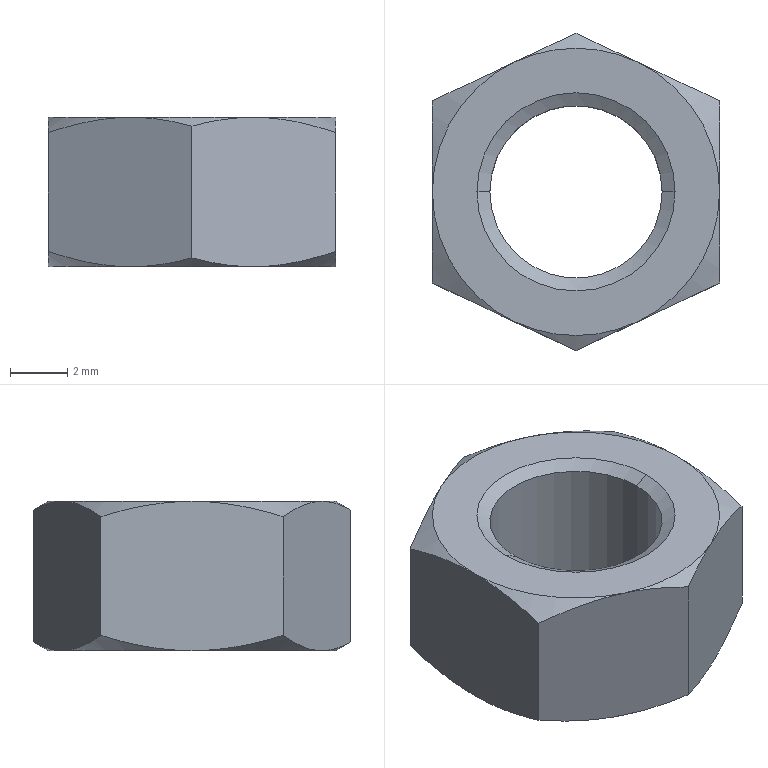Part | SolidWorks | features BaseBody 1 | 1 solid | 26 faces | box 10 x 11.05 x 5.2 mm | volume 300.51 mm3 | cone 16 | plane 8 | cylinder 2 | commonest cylinder face diameters 6 x2
STEP:
#1=CARTESIAN_POINT('',(107.5,-21.,59.86));
#2=VERTEX_POINT('',#1);
#3=CARTESIAN_POINT('',(113.5,-21.,59.86));
#4=VERTEX_POINT('',#3);
#5=CARTESIAN_POINT('',(110.5,-21.,59.86));
#6=DIRECTION('',(0.,0.,1.));
#7=DIRECTION('',(-1.,0.,0.));
#8=AXIS2_PLACEMENT_3D('',#5,#6,#7);
#9=CIRCLE('',#8,3.);
#10=EDGE_CURVE('',#2,#4,#9,.T.);
#11=ORIENTED_EDGE('',*,*,#10,.T.);
#12=CARTESIAN_POINT('',(113.95,-21.,59.6));
#13=VERTEX_POINT('',#12);
#14=CARTESIAN_POINT('',(113.95,-21.,59.6));
#15=DIRECTION('',(0.866,0.,-0.5));
#16=VECTOR('',#15,1000.);
#17=LINE('',#14,#16);
#18=EDGE_CURVE('',#4,#13,#17,.T.);
#19=ORIENTED_EDGE('',*,*,#18,.T.);
#20=CARTESIAN_POINT('',(107.05,-21.,59.6));
#21=VERTEX_POINT('',#20);
#22=CARTESIAN_POINT('',(110.5,-21.,59.6));
#23=DIRECTION('',(0.,0.,-1.));
#24=DIRECTION('',(-1.,0.,0.));
#25=AXIS2_PLACEMENT_3D('',#22,#23,#24);
#26=CIRCLE('',#25,3.45);
#27=EDGE_CURVE('',#13,#21,#26,.T.);
#28=ORIENTED_EDGE('',*,*,#27,.T.);
#29=CARTESIAN_POINT('',(107.05,-21.,59.6));
#30=DIRECTION('',(-0.866,0.,-0.5));
#31=VECTOR('',#30,1000.);
#32=LINE('',#29,#31);
#33=EDGE_CURVE('',#2,#21,#32,.T.);
#34=ORIENTED_EDGE('',*,*,#33,.F.);
#35=EDGE_LOOP('',(#11,#19,#28,#34));
#36=FACE_OUTER_BOUND('',#35,.T.);
#37=CARTESIAN_POINT('',(110.5,-21.,59.6));
#38=DIRECTION('',(0.,0.,-1.));
#39=DIRECTION('',(-1.,0.,0.));
#40=AXIS2_PLACEMENT_3D('',#37,#38,#39);
#41=CONICAL_SURFACE('',#40,3.45,1.047);
#42=ADVANCED_FACE('',(#36),#41,.F.);
#43=CARTESIAN_POINT('',(113.5,-21.,64.54));
#44=VERTEX_POINT('',#43);
#45=CARTESIAN_POINT('',(107.5,-21.,64.54));
#46=VERTEX_POINT('',#45);
#47=CARTESIAN_POINT('',(110.5,-21.,64.54));
#48=DIRECTION('',(0.,0.,-1.));
#49=DIRECTION('',(1.,0.,0.));
#50=AXIS2_PLACEMENT_3D('',#47,#48,#49);
#51=CIRCLE('',#50,3.);
#52=EDGE_CURVE('',#44,#46,#51,.T.);
#53=ORIENTED_EDGE('',*,*,#52,.T.);
#54=CARTESIAN_POINT('',(107.05,-21.,64.8));
#55=VERTEX_POINT('',#54);
#56=CARTESIAN_POINT('',(107.05,-21.,64.8));
#57=DIRECTION('',(-0.866,0.,0.5));
#58=VECTOR('',#57,1000.);
#59=LINE('',#56,#58);
#60=EDGE_CURVE('',#46,#55,#59,.T.);
#61=ORIENTED_EDGE('',*,*,#60,.T.);
#62=CARTESIAN_POINT('',(113.95,-21.,64.8));
#63=VERTEX_POINT('',#62);
#64=CARTESIAN_POINT('',(110.5,-21.,64.8));
#65=DIRECTION('',(0.,0.,1.));
#66=DIRECTION('',(1.,0.,0.));
#67=AXIS2_PLACEMENT_3D('',#64,#65,#66);
#68=CIRCLE('',#67,3.45);
#69=EDGE_CURVE('',#55,#63,#68,.T.);
#70=ORIENTED_EDGE('',*,*,#69,.T.);
#71=CARTESIAN_POINT('',(113.95,-21.,64.8));
#72=DIRECTION('',(0.866,0.,0.5));
#73=VECTOR('',#72,1000.);
#74=LINE('',#71,#73);
#75=EDGE_CURVE('',#44,#63,#74,.T.);
#76=ORIENTED_EDGE('',*,*,#75,.F.);
#77=EDGE_LOOP('',(#53,#61,#70,#76));
#78=FACE_OUTER_BOUND('',#77,.T.);
#79=CARTESIAN_POINT('',(110.5,-21.,64.8));
#80=DIRECTION('',(0.,0.,1.));
#81=DIRECTION('',(1.,0.,0.));
#82=AXIS2_PLACEMENT_3D('',#79,#80,#81);
#83=CONICAL_SURFACE('',#82,3.45,1.047);
#84=ADVANCED_FACE('',(#78),#83,.F.);
#85=ORIENTED_EDGE('',*,*,#52,.F.);
#86=CARTESIAN_POINT('',(113.5,-21.,64.8));
#87=DIRECTION('',(0.,0.,-1.));
#88=VECTOR('',#87,1000.);
#89=LINE('',#86,#88);
#90=EDGE_CURVE('',#44,#4,#89,.T.);
#91=ORIENTED_EDGE('',*,*,#90,.T.);
#92=ORIENTED_EDGE('',*,*,#10,.F.);
#93=CARTESIAN_POINT('',(107.5,-21.,64.8));
#94=DIRECTION('',(0.,0.,-1.));
#95=VECTOR('',#94,1000.);
#96=LINE('',#93,#95);
#97=EDGE_CURVE('',#46,#2,#96,.T.);
#98=ORIENTED_EDGE('',*,*,#97,.F.);
#99=EDGE_LOOP('',(#85,#91,#92,#98));
#100=FACE_OUTER_BOUND('',#99,.T.);
#101=CARTESIAN_POINT('',(110.5,-21.,64.8));
#102=DIRECTION('',(0.,0.,-1.));
#103=DIRECTION('',(-1.,0.,0.));
#104=AXIS2_PLACEMENT_3D('',#101,#102,#103);
#105=CYLINDRICAL_SURFACE('',#104,3.);
#106=ADVANCED_FACE('',(#100),#105,.F.);
#107=CARTESIAN_POINT('',(110.5,-15.475,64.497));
#108=VERTEX_POINT('',#107);
#109=CARTESIAN_POINT('',(108.373,-16.475,64.8));
#110=VERTEX_POINT('',#109);
#111=CARTESIAN_POINT('',(110.5,-15.475,64.497));
#112=CARTESIAN_POINT('',(109.799,-15.805,64.687));
#113=CARTESIAN_POINT('',(109.09,-16.138,64.8));
#114=CARTESIAN_POINT('',(108.373,-16.475,64.8));
#115=B_SPLINE_CURVE_WITH_KNOTS('',3,(#111,#112,#113,#114),.UNSPECIFIED.,.F.,.F.,(4,4),(0.000000225,0.002369),.UNSPECIFIED.);
#116=EDGE_CURVE('',#108,#110,#115,.T.);
#117=ORIENTED_EDGE('',*,*,#116,.F.);
#118=CARTESIAN_POINT('',(110.5,-15.475,59.903));
#119=VERTEX_POINT('',#118);
#120=CARTESIAN_POINT('',(110.5,-15.475,64.8));
#121=DIRECTION('',(0.,0.,-1.));
#122=VECTOR('',#121,1000.);
#123=LINE('',#120,#122);
#124=EDGE_CURVE('',#108,#119,#123,.T.);
#125=ORIENTED_EDGE('',*,*,#124,.T.);
#126=CARTESIAN_POINT('',(108.373,-16.475,59.6));
#127=VERTEX_POINT('',#126);
#128=CARTESIAN_POINT('',(108.373,-16.475,59.6));
#129=CARTESIAN_POINT('',(109.094,-16.136,59.6));
#130=CARTESIAN_POINT('',(109.801,-15.804,59.713));
#131=CARTESIAN_POINT('',(110.5,-15.475,59.903));
#132=B_SPLINE_CURVE_WITH_KNOTS('',3,(#128,#129,#130,#131),.UNSPECIFIED.,.F.,.F.,(4,4),(0.003219,0.005576),.UNSPECIFIED.);
#133=EDGE_CURVE('',#127,#119,#132,.T.);
#134=ORIENTED_EDGE('',*,*,#133,.F.);
#135=CARTESIAN_POINT('',(105.5,-17.826,60.133));
#136=VERTEX_POINT('',#135);
#137=CARTESIAN_POINT('',(105.5,-17.826,60.133));
#138=CARTESIAN_POINT('',(106.436,-17.386,59.813));
#139=CARTESIAN_POINT('',(107.389,-16.938,59.6));
#140=CARTESIAN_POINT('',(108.373,-16.475,59.6));
#141=B_SPLINE_CURVE_WITH_KNOTS('',3,(#137,#138,#139,#140),.UNSPECIFIED.,.F.,.F.,(4,4),(0.000000229,0.003219),.UNSPECIFIED.);
#142=EDGE_CURVE('',#136,#127,#141,.T.);
#143=ORIENTED_EDGE('',*,*,#142,.F.);
#144=CARTESIAN_POINT('',(105.5,-17.826,64.267));
#145=VERTEX_POINT('',#144);
#146=CARTESIAN_POINT('',(105.5,-17.826,64.8));
#147=DIRECTION('',(0.,0.,-1.));
#148=VECTOR('',#147,1000.);
#149=LINE('',#146,#148);
#150=EDGE_CURVE('',#145,#136,#149,.T.);
#151=ORIENTED_EDGE('',*,*,#150,.F.);
#152=CARTESIAN_POINT('',(108.373,-16.475,64.8));
#153=CARTESIAN_POINT('',(108.13,-16.589,64.8));
#154=CARTESIAN_POINT('',(107.885,-16.704,64.787));
#155=CARTESIAN_POINT('',(107.398,-16.933,64.738));
#156=CARTESIAN_POINT('',(107.157,-17.047,64.701));
#157=CARTESIAN_POINT('',(106.439,-17.384,64.561));
#158=CARTESIAN_POINT('',(105.967,-17.606,64.427));
#159=CARTESIAN_POINT('',(105.5,-17.826,64.267));
#160=B_SPLINE_CURVE_WITH_KNOTS('',3,(#152,#153,#154,#155,#156,#157,#158,#159),.UNSPECIFIED.,.F.,.F.,(4,2,2,4),(0.002369,0.00317,0.003971,0.005574),.UNSPECIFIED.);
#161=EDGE_CURVE('',#110,#145,#160,.T.);
#162=ORIENTED_EDGE('',*,*,#161,.F.);
#163=EDGE_LOOP('',(#117,#125,#134,#143,#151,#162));
#164=FACE_OUTER_BOUND('',#163,.T.);
#165=CARTESIAN_POINT('',(105.5,-17.826,64.8));
#166=DIRECTION('',(0.4255,-0.905,0.));
#167=DIRECTION('',(0.905,0.4255,0.));
#168=AXIS2_PLACEMENT_3D('',#165,#166,#167);
#169=PLANE('',#168);
#170=ADVANCED_FACE('',(#164),#169,.F.);
#171=CARTESIAN_POINT('',(105.5,-21.,64.8));
#172=VERTEX_POINT('',#171);
#173=CARTESIAN_POINT('',(105.5,-17.826,64.267));
#174=CARTESIAN_POINT('',(105.5,-18.34,64.427));
#175=CARTESIAN_POINT('',(105.5,-18.861,64.56));
#176=CARTESIAN_POINT('',(105.5,-19.654,64.701));
#177=CARTESIAN_POINT('',(105.5,-19.92,64.737));
#178=CARTESIAN_POINT('',(105.5,-20.458,64.787));
#179=CARTESIAN_POINT('',(105.5,-20.73,64.8));
#180=CARTESIAN_POINT('',(105.5,-21.,64.8));
#181=B_SPLINE_CURVE_WITH_KNOTS('',3,(#173,#174,#175,#176,#177,#178,#179,#180),.UNSPECIFIED.,.F.,.F.,(4,2,2,4),(0.01571,0.01731,0.01812,0.01892),.UNSPECIFIED.);
#182=EDGE_CURVE('',#145,#172,#181,.T.);
#183=ORIENTED_EDGE('',*,*,#182,.F.);
#184=ORIENTED_EDGE('',*,*,#150,.T.);
#185=CARTESIAN_POINT('',(105.5,-21.,59.6));
#186=VERTEX_POINT('',#185);
#187=CARTESIAN_POINT('',(105.5,-21.,59.6));
#188=CARTESIAN_POINT('',(105.5,-20.73,59.6));
#189=CARTESIAN_POINT('',(105.5,-20.458,59.613));
#190=CARTESIAN_POINT('',(105.5,-19.92,59.663));
#191=CARTESIAN_POINT('',(105.5,-19.654,59.699));
#192=CARTESIAN_POINT('',(105.5,-18.861,59.84));
#193=CARTESIAN_POINT('',(105.5,-18.34,59.973));
#194=CARTESIAN_POINT('',(105.5,-17.826,60.133));
#195=B_SPLINE_CURVE_WITH_KNOTS('',3,(#187,#188,#189,#190,#191,#192,#193,#194),.UNSPECIFIED.,.F.,.F.,(4,2,2,4),(0.008694,0.009499,0.0103,0.01192),.UNSPECIFIED.);
#196=EDGE_CURVE('',#186,#136,#195,.T.);
#197=ORIENTED_EDGE('',*,*,#196,.F.);
#198=CARTESIAN_POINT('',(105.5,-24.174,60.133));
#199=VERTEX_POINT('',#198);
#200=CARTESIAN_POINT('',(105.5,-24.174,60.133));
#201=CARTESIAN_POINT('',(105.5,-23.659,59.973));
#202=CARTESIAN_POINT('',(105.5,-23.132,59.838));
#203=CARTESIAN_POINT('',(105.5,-22.074,59.651));
#204=CARTESIAN_POINT('',(105.5,-21.54,59.6));
#205=CARTESIAN_POINT('',(105.5,-21.,59.6));
#206=B_SPLINE_CURVE_WITH_KNOTS('',3,(#200,#201,#202,#203,#204,#205),.UNSPECIFIED.,.F.,.F.,(4,2,4),(0.00547,0.007082,0.008694),.UNSPECIFIED.);
#207=EDGE_CURVE('',#199,#186,#206,.T.);
#208=ORIENTED_EDGE('',*,*,#207,.F.);
#209=CARTESIAN_POINT('',(105.5,-24.174,64.267));
#210=VERTEX_POINT('',#209);
#211=CARTESIAN_POINT('',(105.5,-24.174,64.8));
#212=DIRECTION('',(0.,0.,-1.));
#213=VECTOR('',#212,1000.);
#214=LINE('',#211,#213);
#215=EDGE_CURVE('',#210,#199,#214,.T.);
#216=ORIENTED_EDGE('',*,*,#215,.F.);
#217=CARTESIAN_POINT('',(105.5,-21.,64.8));
#218=CARTESIAN_POINT('',(105.5,-21.54,64.8));
#219=CARTESIAN_POINT('',(105.5,-22.074,64.749));
#220=CARTESIAN_POINT('',(105.5,-23.132,64.562));
#221=CARTESIAN_POINT('',(105.5,-23.659,64.427));
#222=CARTESIAN_POINT('',(105.5,-24.174,64.267));
#223=B_SPLINE_CURVE_WITH_KNOTS('',3,(#217,#218,#219,#220,#221,#222),.UNSPECIFIED.,.F.,.F.,(4,2,4),(0.01892,0.02053,0.02214),.UNSPECIFIED.);
#224=EDGE_CURVE('',#172,#210,#223,.T.);
#225=ORIENTED_EDGE('',*,*,#224,.F.);
#226=EDGE_LOOP('',(#183,#184,#197,#208,#216,#225));
#227=FACE_OUTER_BOUND('',#226,.T.);
#228=CARTESIAN_POINT('',(105.5,-24.174,64.8));
#229=DIRECTION('',(1.,0.,0.));
#230=DIRECTION('',(0.,0.,-1.));
#231=AXIS2_PLACEMENT_3D('',#228,#229,#230);
#232=PLANE('',#231);
#233=ADVANCED_FACE('',(#227),#232,.F.);
#234=CARTESIAN_POINT('',(108.373,-25.525,64.8));
#235=VERTEX_POINT('',#234);
#236=CARTESIAN_POINT('',(105.5,-24.174,64.267));
#237=CARTESIAN_POINT('',(106.436,-24.614,64.587));
#238=CARTESIAN_POINT('',(107.389,-25.062,64.8));
#239=CARTESIAN_POINT('',(108.373,-25.525,64.8));
#240=B_SPLINE_CURVE_WITH_KNOTS('',3,(#236,#237,#238,#239),.UNSPECIFIED.,.F.,.F.,(4,4),(0.000000229,0.003219),.UNSPECIFIED.);
#241=EDGE_CURVE('',#210,#235,#240,.T.);
#242=ORIENTED_EDGE('',*,*,#241,.F.);
#243=ORIENTED_EDGE('',*,*,#215,.T.);
#244=CARTESIAN_POINT('',(108.373,-25.525,59.6));
#245=VERTEX_POINT('',#244);
#246=CARTESIAN_POINT('',(108.373,-25.525,59.6));
#247=CARTESIAN_POINT('',(108.13,-25.411,59.6));
#248=CARTESIAN_POINT('',(107.885,-25.296,59.613));
#249=CARTESIAN_POINT('',(107.398,-25.067,59.662));
#250=CARTESIAN_POINT('',(107.157,-24.953,59.699));
#251=CARTESIAN_POINT('',(106.439,-24.616,59.839));
#252=CARTESIAN_POINT('',(105.967,-24.394,59.973));
#253=CARTESIAN_POINT('',(105.5,-24.174,60.133));
#254=B_SPLINE_CURVE_WITH_KNOTS('',3,(#246,#247,#248,#249,#250,#251,#252,#253),.UNSPECIFIED.,.F.,.F.,(4,2,2,4),(0.002369,0.00317,0.003971,0.005574),.UNSPECIFIED.);
#255=EDGE_CURVE('',#245,#199,#254,.T.);
#256=ORIENTED_EDGE('',*,*,#255,.F.);
#257=CARTESIAN_POINT('',(110.5,-26.525,59.903));
#258=VERTEX_POINT('',#257);
#259=CARTESIAN_POINT('',(110.5,-26.525,59.903));
#260=CARTESIAN_POINT('',(109.799,-26.195,59.713));
#261=CARTESIAN_POINT('',(109.09,-25.862,59.6));
#262=CARTESIAN_POINT('',(108.373,-25.525,59.6));
#263=B_SPLINE_CURVE_WITH_KNOTS('',3,(#259,#260,#261,#262),.UNSPECIFIED.,.F.,.F.,(4,4),(0.000000225,0.002369),.UNSPECIFIED.);
#264=EDGE_CURVE('',#258,#245,#263,.T.);
#265=ORIENTED_EDGE('',*,*,#264,.F.);
#266=CARTESIAN_POINT('',(110.5,-26.525,64.497));
#267=VERTEX_POINT('',#266);
#268=CARTESIAN_POINT('',(110.5,-26.525,64.8));
#269=DIRECTION('',(0.,0.,-1.));
#270=VECTOR('',#269,1000.);
#271=LINE('',#268,#270);
#272=EDGE_CURVE('',#267,#258,#271,.T.);
#273=ORIENTED_EDGE('',*,*,#272,.F.);
#274=CARTESIAN_POINT('',(108.373,-25.525,64.8));
#275=CARTESIAN_POINT('',(109.094,-25.864,64.8));
#276=CARTESIAN_POINT('',(109.801,-26.196,64.687));
#277=CARTESIAN_POINT('',(110.5,-26.525,64.497));
#278=B_SPLINE_CURVE_WITH_KNOTS('',3,(#274,#275,#276,#277),.UNSPECIFIED.,.F.,.F.,(4,4),(0.003219,0.005576),.UNSPECIFIED.);
#279=EDGE_CURVE('',#235,#267,#278,.T.);
#280=ORIENTED_EDGE('',*,*,#279,.F.);
#281=EDGE_LOOP('',(#242,#243,#256,#265,#273,#280));
#282=FACE_OUTER_BOUND('',#281,.T.);
#283=CARTESIAN_POINT('',(105.5,-24.174,64.8));
#284=DIRECTION('',(0.4255,0.905,0.));
#285=DIRECTION('',(-0.905,0.4255,0.));
#286=AXIS2_PLACEMENT_3D('',#283,#284,#285);
#287=PLANE('',#286);
#288=ADVANCED_FACE('',(#282),#287,.F.);
#289=CARTESIAN_POINT('',(112.627,-25.525,64.8));
#290=VERTEX_POINT('',#289);
#291=CARTESIAN_POINT('',(110.5,-26.525,64.497));
#292=CARTESIAN_POINT('',(111.201,-26.195,64.687));
#293=CARTESIAN_POINT('',(111.91,-25.862,64.8));
#294=CARTESIAN_POINT('',(112.627,-25.525,64.8));
#295=B_SPLINE_CURVE_WITH_KNOTS('',3,(#291,#292,#293,#294),.UNSPECIFIED.,.F.,.F.,(4,4),(0.000000225,0.002369),.UNSPECIFIED.);
#296=EDGE_CURVE('',#267,#290,#295,.T.);
#297=ORIENTED_EDGE('',*,*,#296,.F.);
#298=ORIENTED_EDGE('',*,*,#272,.T.);
#299=CARTESIAN_POINT('',(112.627,-25.525,59.6));
#300=VERTEX_POINT('',#299);
#301=CARTESIAN_POINT('',(112.627,-25.525,59.6));
#302=CARTESIAN_POINT('',(111.906,-25.864,59.6));
#303=CARTESIAN_POINT('',(111.199,-26.196,59.713));
#304=CARTESIAN_POINT('',(110.5,-26.525,59.903));
#305=B_SPLINE_CURVE_WITH_KNOTS('',3,(#301,#302,#303,#304),.UNSPECIFIED.,.F.,.F.,(4,4),(0.003219,0.005576),.UNSPECIFIED.);
#306=EDGE_CURVE('',#300,#258,#305,.T.);
#307=ORIENTED_EDGE('',*,*,#306,.F.);
#308=CARTESIAN_POINT('',(115.5,-24.174,60.133));
#309=VERTEX_POINT('',#308);
#310=CARTESIAN_POINT('',(115.5,-24.174,60.133));
#311=CARTESIAN_POINT('',(114.564,-24.614,59.813));
#312=CARTESIAN_POINT('',(113.611,-25.062,59.6));
#313=CARTESIAN_POINT('',(112.627,-25.525,59.6));
#314=B_SPLINE_CURVE_WITH_KNOTS('',3,(#310,#311,#312,#313),.UNSPECIFIED.,.F.,.F.,(4,4),(0.000000229,0.003219),.UNSPECIFIED.);
#315=EDGE_CURVE('',#309,#300,#314,.T.);
#316=ORIENTED_EDGE('',*,*,#315,.F.);
#317=CARTESIAN_POINT('',(115.5,-24.174,64.267));
#318=VERTEX_POINT('',#317);
#319=CARTESIAN_POINT('',(115.5,-24.174,64.8));
#320=DIRECTION('',(0.,0.,-1.));
#321=VECTOR('',#320,1000.);
#322=LINE('',#319,#321);
#323=EDGE_CURVE('',#318,#309,#322,.T.);
#324=ORIENTED_EDGE('',*,*,#323,.F.);
#325=CARTESIAN_POINT('',(112.627,-25.525,64.8));
#326=CARTESIAN_POINT('',(112.87,-25.411,64.8));
#327=CARTESIAN_POINT('',(113.115,-25.296,64.787));
#328=CARTESIAN_POINT('',(113.602,-25.067,64.738));
#329=CARTESIAN_POINT('',(113.843,-24.953,64.701));
#330=CARTESIAN_POINT('',(114.561,-24.616,64.561));
#331=CARTESIAN_POINT('',(115.033,-24.394,64.427));
#332=CARTESIAN_POINT('',(115.5,-24.174,64.267));
#333=B_SPLINE_CURVE_WITH_KNOTS('',3,(#325,#326,#327,#328,#329,#330,#331,#332),.UNSPECIFIED.,.F.,.F.,(4,2,2,4),(0.002369,0.00317,0.003971,0.005574),.UNSPECIFIED.);
#334=EDGE_CURVE('',#290,#318,#333,.T.);
#335=ORIENTED_EDGE('',*,*,#334,.F.);
#336=EDGE_LOOP('',(#297,#298,#307,#316,#324,#335));
#337=FACE_OUTER_BOUND('',#336,.T.);
#338=CARTESIAN_POINT('',(115.5,-24.174,64.8));
#339=DIRECTION('',(-0.4255,0.905,0.));
#340=DIRECTION('',(-0.905,-0.4255,0.));
#341=AXIS2_PLACEMENT_3D('',#338,#339,#340);
#342=PLANE('',#341);
#343=ADVANCED_FACE('',(#337),#342,.F.);
#344=CARTESIAN_POINT('',(115.5,-21.,64.8));
#345=VERTEX_POINT('',#344);
#346=CARTESIAN_POINT('',(115.5,-24.174,64.267));
#347=CARTESIAN_POINT('',(115.5,-23.659,64.427));
#348=CARTESIAN_POINT('',(115.5,-23.132,64.562));
#349=CARTESIAN_POINT('',(115.5,-22.074,64.749));
#350=CARTESIAN_POINT('',(115.5,-21.54,64.8));
#351=CARTESIAN_POINT('',(115.5,-21.,64.8));
#352=B_SPLINE_CURVE_WITH_KNOTS('',3,(#346,#347,#348,#349,#350,#351),.UNSPECIFIED.,.F.,.F.,(4,2,4),(0.00547,0.007082,0.008694),.UNSPECIFIED.);
#353=EDGE_CURVE('',#318,#345,#352,.T.);
#354=ORIENTED_EDGE('',*,*,#353,.F.);
#355=ORIENTED_EDGE('',*,*,#323,.T.);
#356=CARTESIAN_POINT('',(115.5,-21.,59.6));
#357=VERTEX_POINT('',#356);
#358=CARTESIAN_POINT('',(115.5,-21.,59.6));
#359=CARTESIAN_POINT('',(115.5,-21.54,59.6));
#360=CARTESIAN_POINT('',(115.5,-22.074,59.651));
#361=CARTESIAN_POINT('',(115.5,-23.132,59.838));
#362=CARTESIAN_POINT('',(115.5,-23.659,59.973));
#363=CARTESIAN_POINT('',(115.5,-24.174,60.133));
#364=B_SPLINE_CURVE_WITH_KNOTS('',3,(#358,#359,#360,#361,#362,#363),.UNSPECIFIED.,.F.,.F.,(4,2,4),(0.01892,0.02053,0.02214),.UNSPECIFIED.);
#365=EDGE_CURVE('',#357,#309,#364,.T.);
#366=ORIENTED_EDGE('',*,*,#365,.F.);
#367=CARTESIAN_POINT('',(115.5,-17.826,60.133));
#368=VERTEX_POINT('',#367);
#369=CARTESIAN_POINT('',(115.5,-17.826,60.133));
#370=CARTESIAN_POINT('',(115.5,-18.34,59.973));
#371=CARTESIAN_POINT('',(115.5,-18.861,59.84));
#372=CARTESIAN_POINT('',(115.5,-19.654,59.699));
#373=CARTESIAN_POINT('',(115.5,-19.92,59.663));
#374=CARTESIAN_POINT('',(115.5,-20.458,59.613));
#375=CARTESIAN_POINT('',(115.5,-20.73,59.6));
#376=CARTESIAN_POINT('',(115.5,-21.,59.6));
#377=B_SPLINE_CURVE_WITH_KNOTS('',3,(#369,#370,#371,#372,#373,#374,#375,#376),.UNSPECIFIED.,.F.,.F.,(4,2,2,4),(0.01571,0.01731,0.01812,0.01892),.UNSPECIFIED.);
#378=EDGE_CURVE('',#368,#357,#377,.T.);
#379=ORIENTED_EDGE('',*,*,#378,.F.);
#380=CARTESIAN_POINT('',(115.5,-17.826,64.267));
#381=VERTEX_POINT('',#380);
#382=CARTESIAN_POINT('',(115.5,-17.826,64.8));
#383=DIRECTION('',(0.,0.,-1.));
#384=VECTOR('',#383,1000.);
#385=LINE('',#382,#384);
#386=EDGE_CURVE('',#381,#368,#385,.T.);
#387=ORIENTED_EDGE('',*,*,#386,.F.);
#388=CARTESIAN_POINT('',(115.5,-21.,64.8));
#389=CARTESIAN_POINT('',(115.5,-20.73,64.8));
#390=CARTESIAN_POINT('',(115.5,-20.458,64.787));
#391=CARTESIAN_POINT('',(115.5,-19.92,64.737));
#392=CARTESIAN_POINT('',(115.5,-19.654,64.701));
#393=CARTESIAN_POINT('',(115.5,-18.861,64.56));
#394=CARTESIAN_POINT('',(115.5,-18.34,64.427));
#395=CARTESIAN_POINT('',(115.5,-17.826,64.267));
#396=B_SPLINE_CURVE_WITH_KNOTS('',3,(#388,#389,#390,#391,#392,#393,#394,#395),.UNSPECIFIED.,.F.,.F.,(4,2,2,4),(0.008694,0.009499,0.0103,0.01192),.UNSPECIFIED.);
#397=EDGE_CURVE('',#345,#381,#396,.T.);
#398=ORIENTED_EDGE('',*,*,#397,.F.);
#399=EDGE_LOOP('',(#354,#355,#366,#379,#387,#398));
#400=FACE_OUTER_BOUND('',#399,.T.);
#401=CARTESIAN_POINT('',(115.5,-24.174,64.8));
#402=DIRECTION('',(-1.,0.,0.));
#403=DIRECTION('',(0.,0.,1.));
#404=AXIS2_PLACEMENT_3D('',#401,#402,#403);
#405=PLANE('',#404);
#406=ADVANCED_FACE('',(#400),#405,.F.);
#407=CARTESIAN_POINT('',(112.627,-16.475,64.8));
#408=VERTEX_POINT('',#407);
#409=CARTESIAN_POINT('',(115.5,-17.826,64.267));
#410=CARTESIAN_POINT('',(114.564,-17.386,64.587));
#411=CARTESIAN_POINT('',(113.611,-16.938,64.8));
#412=CARTESIAN_POINT('',(112.627,-16.475,64.8));
#413=B_SPLINE_CURVE_WITH_KNOTS('',3,(#409,#410,#411,#412),.UNSPECIFIED.,.F.,.F.,(4,4),(0.000000229,0.003219),.UNSPECIFIED.);
#414=EDGE_CURVE('',#381,#408,#413,.T.);
#415=ORIENTED_EDGE('',*,*,#414,.F.);
#416=ORIENTED_EDGE('',*,*,#386,.T.);
#417=CARTESIAN_POINT('',(112.627,-16.475,59.6));
#418=VERTEX_POINT('',#417);
#419=CARTESIAN_POINT('',(112.627,-16.475,59.6));
#420=CARTESIAN_POINT('',(112.87,-16.589,59.6));
#421=CARTESIAN_POINT('',(113.115,-16.704,59.613));
#422=CARTESIAN_POINT('',(113.602,-16.933,59.662));
#423=CARTESIAN_POINT('',(113.843,-17.047,59.699));
#424=CARTESIAN_POINT('',(114.561,-17.384,59.839));
#425=CARTESIAN_POINT('',(115.033,-17.606,59.973));
#426=CARTESIAN_POINT('',(115.5,-17.826,60.133));
#427=B_SPLINE_CURVE_WITH_KNOTS('',3,(#419,#420,#421,#422,#423,#424,#425,#426),.UNSPECIFIED.,.F.,.F.,(4,2,2,4),(0.002369,0.00317,0.003971,0.005574),.UNSPECIFIED.);
#428=EDGE_CURVE('',#418,#368,#427,.T.);
#429=ORIENTED_EDGE('',*,*,#428,.F.);
#430=CARTESIAN_POINT('',(110.5,-15.475,59.903));
#431=CARTESIAN_POINT('',(111.201,-15.805,59.713));
#432=CARTESIAN_POINT('',(111.91,-16.138,59.6));
#433=CARTESIAN_POINT('',(112.627,-16.475,59.6));
#434=B_SPLINE_CURVE_WITH_KNOTS('',3,(#430,#431,#432,#433),.UNSPECIFIED.,.F.,.F.,(4,4),(0.000000225,0.002369),.UNSPECIFIED.);
#435=EDGE_CURVE('',#119,#418,#434,.T.);
#436=ORIENTED_EDGE('',*,*,#435,.F.);
#437=ORIENTED_EDGE('',*,*,#124,.F.);
#438=CARTESIAN_POINT('',(112.627,-16.475,64.8));
#439=CARTESIAN_POINT('',(111.906,-16.136,64.8));
#440=CARTESIAN_POINT('',(111.199,-15.804,64.687));
#441=CARTESIAN_POINT('',(110.5,-15.475,64.497));
#442=B_SPLINE_CURVE_WITH_KNOTS('',3,(#438,#439,#440,#441),.UNSPECIFIED.,.F.,.F.,(4,4),(0.003219,0.005576),.UNSPECIFIED.);
#443=EDGE_CURVE('',#408,#108,#442,.T.);
#444=ORIENTED_EDGE('',*,*,#443,.F.);
#445=EDGE_LOOP('',(#415,#416,#429,#436,#437,#444));
#446=FACE_OUTER_BOUND('',#445,.T.);
#447=CARTESIAN_POINT('',(115.5,-17.826,64.8));
#448=DIRECTION('',(-0.4255,-0.905,0.));
#449=DIRECTION('',(0.905,-0.4255,0.));
#450=AXIS2_PLACEMENT_3D('',#447,#448,#449);
#451=PLANE('',#450);
#452=ADVANCED_FACE('',(#446),#451,.F.);
#453=CARTESIAN_POINT('',(110.5,-21.,64.8));
#454=DIRECTION('',(0.,0.,1.));
#455=DIRECTION('',(1.,0.,0.));
#456=AXIS2_PLACEMENT_3D('',#453,#454,#455);
#457=CIRCLE('',#456,3.45);
#458=EDGE_CURVE('',#63,#55,#457,.T.);
#459=ORIENTED_EDGE('',*,*,#458,.F.);
#460=ORIENTED_EDGE('',*,*,#69,.F.);
#461=EDGE_LOOP('',(#459,#460));
#462=FACE_BOUND('',#461,.T.);
#463=CARTESIAN_POINT('',(110.5,-21.,64.8));
#464=DIRECTION('',(0.,0.,1.));
#465=DIRECTION('',(1.,0.,0.));
#466=AXIS2_PLACEMENT_3D('',#463,#464,#465);
#467=CIRCLE('',#466,5.);
#468=EDGE_CURVE('',#290,#345,#467,.T.);
#469=ORIENTED_EDGE('',*,*,#468,.T.);
#470=CARTESIAN_POINT('',(110.5,-21.,64.8));
#471=DIRECTION('',(0.,0.,1.));
#472=DIRECTION('',(1.,0.,0.));
#473=AXIS2_PLACEMENT_3D('',#470,#471,#472);
#474=CIRCLE('',#473,5.);
#475=EDGE_CURVE('',#345,#408,#474,.T.);
#476=ORIENTED_EDGE('',*,*,#475,.T.);
#477=CARTESIAN_POINT('',(110.5,-21.,64.8));
#478=DIRECTION('',(0.,0.,1.));
#479=DIRECTION('',(1.,0.,0.));
#480=AXIS2_PLACEMENT_3D('',#477,#478,#479);
#481=CIRCLE('',#480,5.);
#482=EDGE_CURVE('',#408,#110,#481,.T.);
#483=ORIENTED_EDGE('',*,*,#482,.T.);
#484=CARTESIAN_POINT('',(110.5,-21.,64.8));
#485=DIRECTION('',(0.,0.,1.));
#486=DIRECTION('',(1.,0.,0.));
#487=AXIS2_PLACEMENT_3D('',#484,#485,#486);
#488=CIRCLE('',#487,5.);
#489=EDGE_CURVE('',#110,#172,#488,.T.);
#490=ORIENTED_EDGE('',*,*,#489,.T.);
#491=CARTESIAN_POINT('',(110.5,-21.,64.8));
#492=DIRECTION('',(0.,0.,1.));
#493=DIRECTION('',(1.,0.,0.));
#494=AXIS2_PLACEMENT_3D('',#491,#492,#493);
#495=CIRCLE('',#494,5.);
#496=EDGE_CURVE('',#172,#235,#495,.T.);
#497=ORIENTED_EDGE('',*,*,#496,.T.);
#498=CARTESIAN_POINT('',(110.5,-21.,64.8));
#499=DIRECTION('',(0.,0.,1.));
#500=DIRECTION('',(1.,0.,0.));
#501=AXIS2_PLACEMENT_3D('',#498,#499,#500);
#502=CIRCLE('',#501,5.);
#503=EDGE_CURVE('',#235,#290,#502,.T.);
#504=ORIENTED_EDGE('',*,*,#503,.T.);
#505=EDGE_LOOP('',(#469,#476,#483,#490,#497,#504));
#506=FACE_OUTER_BOUND('',#505,.T.);
#507=CARTESIAN_POINT('',(115.5,-13.124,64.8));
#508=DIRECTION('',(0.,0.,1.));
#509=DIRECTION('',(1.,0.,0.));
#510=AXIS2_PLACEMENT_3D('',#507,#508,#509);
#511=PLANE('',#510);
#512=ADVANCED_FACE('',(#462,#506),#511,.T.);
#513=CARTESIAN_POINT('',(110.5,-21.,59.6));
#514=DIRECTION('',(0.,0.,-1.));
#515=DIRECTION('',(-1.,0.,0.));
#516=AXIS2_PLACEMENT_3D('',#513,#514,#515);
#517=CIRCLE('',#516,3.45);
#518=EDGE_CURVE('',#21,#13,#517,.T.);
#519=ORIENTED_EDGE('',*,*,#518,.F.);
#520=ORIENTED_EDGE('',*,*,#27,.F.);
#521=EDGE_LOOP('',(#519,#520));
#522=FACE_BOUND('',#521,.T.);
#523=CARTESIAN_POINT('',(110.5,-21.,59.6));
#524=DIRECTION('',(0.,0.,-1.));
#525=DIRECTION('',(-1.,0.,0.));
#526=AXIS2_PLACEMENT_3D('',#523,#524,#525);
#527=CIRCLE('',#526,5.);
#528=EDGE_CURVE('',#418,#357,#527,.T.);
#529=ORIENTED_EDGE('',*,*,#528,.T.);
#530=CARTESIAN_POINT('',(110.5,-21.,59.6));
#531=DIRECTION('',(0.,0.,-1.));
#532=DIRECTION('',(-1.,0.,0.));
#533=AXIS2_PLACEMENT_3D('',#530,#531,#532);
#534=CIRCLE('',#533,5.);
#535=EDGE_CURVE('',#357,#300,#534,.T.);
#536=ORIENTED_EDGE('',*,*,#535,.T.);
#537=CARTESIAN_POINT('',(110.5,-21.,59.6));
#538=DIRECTION('',(0.,0.,-1.));
#539=DIRECTION('',(-1.,0.,0.));
#540=AXIS2_PLACEMENT_3D('',#537,#538,#539);
#541=CIRCLE('',#540,5.);
#542=EDGE_CURVE('',#300,#245,#541,.T.);
#543=ORIENTED_EDGE('',*,*,#542,.T.);
#544=CARTESIAN_POINT('',(110.5,-21.,59.6));
#545=DIRECTION('',(0.,0.,-1.));
#546=DIRECTION('',(-1.,0.,0.));
#547=AXIS2_PLACEMENT_3D('',#544,#545,#546);
#548=CIRCLE('',#547,5.);
#549=EDGE_CURVE('',#245,#186,#548,.T.);
#550=ORIENTED_EDGE('',*,*,#549,.T.);
#551=CARTESIAN_POINT('',(110.5,-21.,59.6));
#552=DIRECTION('',(0.,0.,-1.));
#553=DIRECTION('',(-1.,0.,0.));
#554=AXIS2_PLACEMENT_3D('',#551,#552,#553);
#555=CIRCLE('',#554,5.);
#556=EDGE_CURVE('',#186,#127,#555,.T.);
#557=ORIENTED_EDGE('',*,*,#556,.T.);
#558=CARTESIAN_POINT('',(110.5,-21.,59.6));
#559=DIRECTION('',(0.,0.,-1.));
#560=DIRECTION('',(-1.,0.,0.));
#561=AXIS2_PLACEMENT_3D('',#558,#559,#560);
#562=CIRCLE('',#561,5.);
#563=EDGE_CURVE('',#127,#418,#562,.T.);
#564=ORIENTED_EDGE('',*,*,#563,.T.);
#565=EDGE_LOOP('',(#529,#536,#543,#550,#557,#564));
#566=FACE_OUTER_BOUND('',#565,.T.);
#567=CARTESIAN_POINT('',(115.5,-13.124,59.6));
#568=DIRECTION('',(0.,0.,1.));
#569=DIRECTION('',(1.,0.,0.));
#570=AXIS2_PLACEMENT_3D('',#567,#568,#569);
#571=PLANE('',#570);
#572=ADVANCED_FACE('',(#522,#566),#571,.F.);
#573=ORIENTED_EDGE('',*,*,#90,.F.);
#574=CARTESIAN_POINT('',(110.5,-21.,64.54));
#575=DIRECTION('',(0.,0.,-1.));
#576=DIRECTION('',(1.,0.,0.));
#577=AXIS2_PLACEMENT_3D('',#574,#575,#576);
#578=CIRCLE('',#577,3.);
#579=EDGE_CURVE('',#46,#44,#578,.T.);
#580=ORIENTED_EDGE('',*,*,#579,.F.);
#581=ORIENTED_EDGE('',*,*,#97,.T.);
#582=CARTESIAN_POINT('',(110.5,-21.,59.86));
#583=DIRECTION('',(0.,0.,1.));
#584=DIRECTION('',(-1.,0.,0.));
#585=AXIS2_PLACEMENT_3D('',#582,#583,#584);
#586=CIRCLE('',#585,3.);
#587=EDGE_CURVE('',#4,#2,#586,.T.);
#588=ORIENTED_EDGE('',*,*,#587,.F.);
#589=EDGE_LOOP('',(#573,#580,#581,#588));
#590=FACE_OUTER_BOUND('',#589,.T.);
#591=CARTESIAN_POINT('',(110.5,-21.,64.8));
#592=DIRECTION('',(0.,0.,-1.));
#593=DIRECTION('',(-1.,0.,0.));
#594=AXIS2_PLACEMENT_3D('',#591,#592,#593);
#595=CYLINDRICAL_SURFACE('',#594,3.);
#596=ADVANCED_FACE('',(#590),#595,.F.);
#597=ORIENTED_EDGE('',*,*,#378,.T.);
#598=ORIENTED_EDGE('',*,*,#528,.F.);
#599=ORIENTED_EDGE('',*,*,#428,.T.);
#600=EDGE_LOOP('',(#597,#598,#599));
#601=FACE_OUTER_BOUND('',#600,.T.);
#602=CARTESIAN_POINT('',(110.5,-21.,59.6));
#603=DIRECTION('',(0.,0.,1.));
#604=DIRECTION('',(-1.,0.,0.));
#605=AXIS2_PLACEMENT_3D('',#602,#603,#604);
#606=CONICAL_SURFACE('',#605,5.,1.047);
#607=ADVANCED_FACE('',(#601),#606,.T.);
#608=ORIENTED_EDGE('',*,*,#133,.T.);
#609=ORIENTED_EDGE('',*,*,#435,.T.);
#610=ORIENTED_EDGE('',*,*,#563,.F.);
#611=EDGE_LOOP('',(#608,#609,#610));
#612=FACE_OUTER_BOUND('',#611,.T.);
#613=CARTESIAN_POINT('',(110.5,-21.,59.6));
#614=DIRECTION('',(0.,0.,1.));
#615=DIRECTION('',(-1.,0.,0.));
#616=AXIS2_PLACEMENT_3D('',#613,#614,#615);
#617=CONICAL_SURFACE('',#616,5.,1.047);
#618=ADVANCED_FACE('',(#612),#617,.T.);
#619=ORIENTED_EDGE('',*,*,#315,.T.);
#620=ORIENTED_EDGE('',*,*,#535,.F.);
#621=ORIENTED_EDGE('',*,*,#365,.T.);
#622=EDGE_LOOP('',(#619,#620,#621));
#623=FACE_OUTER_BOUND('',#622,.T.);
#624=CARTESIAN_POINT('',(110.5,-21.,59.6));
#625=DIRECTION('',(0.,0.,1.));
#626=DIRECTION('',(-1.,0.,0.));
#627=AXIS2_PLACEMENT_3D('',#624,#625,#626);
#628=CONICAL_SURFACE('',#627,5.,1.047);
#629=ADVANCED_FACE('',(#623),#628,.T.);
#630=ORIENTED_EDGE('',*,*,#264,.T.);
#631=ORIENTED_EDGE('',*,*,#542,.F.);
#632=ORIENTED_EDGE('',*,*,#306,.T.);
#633=EDGE_LOOP('',(#630,#631,#632));
#634=FACE_OUTER_BOUND('',#633,.T.);
#635=CARTESIAN_POINT('',(110.5,-21.,59.6));
#636=DIRECTION('',(0.,0.,1.));
#637=DIRECTION('',(-1.,0.,0.));
#638=AXIS2_PLACEMENT_3D('',#635,#636,#637);
#639=CONICAL_SURFACE('',#638,5.,1.047);
#640=ADVANCED_FACE('',(#634),#639,.T.);
#641=ORIENTED_EDGE('',*,*,#255,.T.);
#642=ORIENTED_EDGE('',*,*,#207,.T.);
#643=ORIENTED_EDGE('',*,*,#549,.F.);
#644=EDGE_LOOP('',(#641,#642,#643));
#645=FACE_OUTER_BOUND('',#644,.T.);
#646=CARTESIAN_POINT('',(110.5,-21.,59.6));
#647=DIRECTION('',(0.,0.,1.));
#648=DIRECTION('',(-1.,0.,0.));
#649=AXIS2_PLACEMENT_3D('',#646,#647,#648);
#650=CONICAL_SURFACE('',#649,5.,1.047);
#651=ADVANCED_FACE('',(#645),#650,.T.);
#652=ORIENTED_EDGE('',*,*,#196,.T.);
#653=ORIENTED_EDGE('',*,*,#142,.T.);
#654=ORIENTED_EDGE('',*,*,#556,.F.);
#655=EDGE_LOOP('',(#652,#653,#654));
#656=FACE_OUTER_BOUND('',#655,.T.);
#657=CARTESIAN_POINT('',(110.5,-21.,59.6));
#658=DIRECTION('',(0.,0.,1.));
#659=DIRECTION('',(-1.,0.,0.));
#660=AXIS2_PLACEMENT_3D('',#657,#658,#659);
#661=CONICAL_SURFACE('',#660,5.,1.047);
#662=ADVANCED_FACE('',(#656),#661,.T.);
#663=ORIENTED_EDGE('',*,*,#334,.T.);
#664=ORIENTED_EDGE('',*,*,#353,.T.);
#665=ORIENTED_EDGE('',*,*,#468,.F.);
#666=EDGE_LOOP('',(#663,#664,#665));
#667=FACE_OUTER_BOUND('',#666,.T.);
#668=CARTESIAN_POINT('',(110.5,-21.,64.8));
#669=DIRECTION('',(0.,0.,-1.));
#670=DIRECTION('',(1.,0.,0.));
#671=AXIS2_PLACEMENT_3D('',#668,#669,#670);
#672=CONICAL_SURFACE('',#671,5.,1.047);
#673=ADVANCED_FACE('',(#667),#672,.T.);
#674=ORIENTED_EDGE('',*,*,#279,.T.);
#675=ORIENTED_EDGE('',*,*,#296,.T.);
#676=ORIENTED_EDGE('',*,*,#503,.F.);
#677=EDGE_LOOP('',(#674,#675,#676));
#678=FACE_OUTER_BOUND('',#677,.T.);
#679=CARTESIAN_POINT('',(110.5,-21.,64.8));
#680=DIRECTION('',(0.,0.,-1.));
#681=DIRECTION('',(1.,0.,0.));
#682=AXIS2_PLACEMENT_3D('',#679,#680,#681);
#683=CONICAL_SURFACE('',#682,5.,1.047);
#684=ADVANCED_FACE('',(#678),#683,.T.);
#685=ORIENTED_EDGE('',*,*,#224,.T.);
#686=ORIENTED_EDGE('',*,*,#241,.T.);
#687=ORIENTED_EDGE('',*,*,#496,.F.);
#688=EDGE_LOOP('',(#685,#686,#687));
#689=FACE_OUTER_BOUND('',#688,.T.);
#690=CARTESIAN_POINT('',(110.5,-21.,64.8));
#691=DIRECTION('',(0.,0.,-1.));
#692=DIRECTION('',(1.,0.,0.));
#693=AXIS2_PLACEMENT_3D('',#690,#691,#692);
#694=CONICAL_SURFACE('',#693,5.,1.047);
#695=ADVANCED_FACE('',(#689),#694,.T.);
#696=ORIENTED_EDGE('',*,*,#161,.T.);
#697=ORIENTED_EDGE('',*,*,#182,.T.);
#698=ORIENTED_EDGE('',*,*,#489,.F.);
#699=EDGE_LOOP('',(#696,#697,#698));
#700=FACE_OUTER_BOUND('',#699,.T.);
#701=CARTESIAN_POINT('',(110.5,-21.,64.8));
#702=DIRECTION('',(0.,0.,-1.));
#703=DIRECTION('',(1.,0.,0.));
#704=AXIS2_PLACEMENT_3D('',#701,#702,#703);
#705=CONICAL_SURFACE('',#704,5.,1.047);
#706=ADVANCED_FACE('',(#700),#705,.T.);
#707=ORIENTED_EDGE('',*,*,#116,.T.);
#708=ORIENTED_EDGE('',*,*,#482,.F.);
#709=ORIENTED_EDGE('',*,*,#443,.T.);
#710=EDGE_LOOP('',(#707,#708,#709));
#711=FACE_OUTER_BOUND('',#710,.T.);
#712=CARTESIAN_POINT('',(110.5,-21.,64.8));
#713=DIRECTION('',(0.,0.,-1.));
#714=DIRECTION('',(1.,0.,0.));
#715=AXIS2_PLACEMENT_3D('',#712,#713,#714);
#716=CONICAL_SURFACE('',#715,5.,1.047);
#717=ADVANCED_FACE('',(#711),#716,.T.);
#718=ORIENTED_EDGE('',*,*,#397,.T.);
#719=ORIENTED_EDGE('',*,*,#414,.T.);
#720=ORIENTED_EDGE('',*,*,#475,.F.);
#721=EDGE_LOOP('',(#718,#719,#720));
#722=FACE_OUTER_BOUND('',#721,.T.);
#723=CARTESIAN_POINT('',(110.5,-21.,64.8));
#724=DIRECTION('',(0.,0.,-1.));
#725=DIRECTION('',(1.,0.,0.));
#726=AXIS2_PLACEMENT_3D('',#723,#724,#725);
#727=CONICAL_SURFACE('',#726,5.,1.047);
#728=ADVANCED_FACE('',(#722),#727,.T.);
#729=ORIENTED_EDGE('',*,*,#60,.F.);
#730=ORIENTED_EDGE('',*,*,#579,.T.);
#731=ORIENTED_EDGE('',*,*,#75,.T.);
#732=ORIENTED_EDGE('',*,*,#458,.T.);
#733=EDGE_LOOP('',(#729,#730,#731,#732));
#734=FACE_OUTER_BOUND('',#733,.T.);
#735=CARTESIAN_POINT('',(110.5,-21.,64.8));
#736=DIRECTION('',(0.,0.,1.));
#737=DIRECTION('',(1.,0.,0.));
#738=AXIS2_PLACEMENT_3D('',#735,#736,#737);
#739=CONICAL_SURFACE('',#738,3.45,1.047);
#740=ADVANCED_FACE('',(#734),#739,.F.);
#741=ORIENTED_EDGE('',*,*,#18,.F.);
#742=ORIENTED_EDGE('',*,*,#587,.T.);
#743=ORIENTED_EDGE('',*,*,#33,.T.);
#744=ORIENTED_EDGE('',*,*,#518,.T.);
#745=EDGE_LOOP('',(#741,#742,#743,#744));
#746=FACE_OUTER_BOUND('',#745,.T.);
#747=CARTESIAN_POINT('',(110.5,-21.,59.6));
#748=DIRECTION('',(0.,0.,-1.));
#749=DIRECTION('',(-1.,0.,0.));
#750=AXIS2_PLACEMENT_3D('',#747,#748,#749);
#751=CONICAL_SURFACE('',#750,3.45,1.047);
#752=ADVANCED_FACE('',(#746),#751,.F.);
#753=CLOSED_SHELL('',(#42,#84,#106,#170,#233,#288,#343,#406,#452,#512,#572,#596,#607,#618,#629,#640,#651,#662,#673,#684,#695,#706,#717,#728,#740,#752));
#754=MANIFOLD_SOLID_BREP('',#753);
#755=CARTESIAN_POINT('',(0.,0.,0.));
#756=DIRECTION('',(0.,0.,1.));
#757=DIRECTION('',(1.,0.,0.));
#758=AXIS2_PLACEMENT_3D('',#755,#756,#757);
#759=(LENGTH_UNIT()NAMED_UNIT(*)SI_UNIT(.MILLI.,.METRE.));
#760=UNCERTAINTY_MEASURE_WITH_UNIT(LENGTH_MEASURE(0.00001),#759,'','');
#761=(NAMED_UNIT(*)PLANE_ANGLE_UNIT()SI_UNIT($,.RADIAN.));
#762=(NAMED_UNIT(*)SI_UNIT($,.STERADIAN.)SOLID_ANGLE_UNIT());
#763=(GEOMETRIC_REPRESENTATION_CONTEXT(3)GLOBAL_UNCERTAINTY_ASSIGNED_CONTEXT((#760))GLOBAL_UNIT_ASSIGNED_CONTEXT((#759,#761,#762))REPRESENTATION_CONTEXT('',''));
#764=ADVANCED_BREP_SHAPE_REPRESENTATION('',(#754,#758),#763);